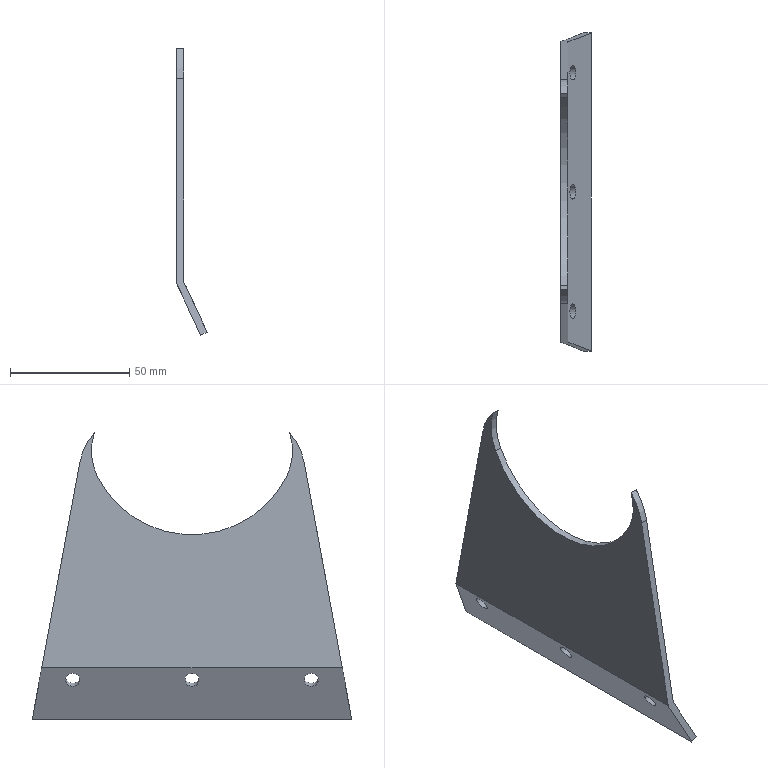Part | STEP file | 1-57.4 | 1 solid | 15 faces | box 12.749 x 134.024 x 120.156 mm | volume 31818 mm3 | cylinder 8 | plane 7 | commonest cylinder face diameters 6 x3 48 x2 51.19 x2 89 x1
STEP:
#1=CARTESIAN_POINT('',(0.,0.,0.));
#2=DIRECTION('',(0.,0.,1.));
#3=DIRECTION('',(1.,0.,0.));
#4=AXIS2_PLACEMENT_3D('',#1,#2,#3);
#5=CARTESIAN_POINT('',(0.,47.074,4.632));
#6=VERTEX_POINT('',#5);
#7=CARTESIAN_POINT('',(3.,47.074,4.632));
#8=VERTEX_POINT('',#7);
#9=CARTESIAN_POINT('',(0.,47.074,4.632));
#10=DIRECTION('',(1.,0.,0.));
#11=VECTOR('',#10,1.);
#12=LINE('',#9,#11);
#13=CARTESIAN_POINT('',(0.,57.043,-49.216));
#14=DIRECTION('',(0.,0.9833,0.182));
#15=DIRECTION('',(0.,-0.182,0.9833));
#16=AXIS2_PLACEMENT_3D('',#13,#14,#15);
#17=PLANE('',#16);
#18=CARTESIAN_POINT('',(54.763,0.));
#19=DIRECTION('',(0.,1.));
#20=VECTOR('',#19,1.);
#21=LINE('',#18,#20);
#22=(GEOMETRIC_REPRESENTATION_CONTEXT(2)PARAMETRIC_REPRESENTATION_CONTEXT()REPRESENTATION_CONTEXT('',''));
#23=DEFINITIONAL_REPRESENTATION('',(#21),#22);
#24=PCURVE('',#17,#23);
#25=CARTESIAN_POINT('',(-80.,21.907,-0.02707));
#26=DIRECTION('',(1.,0.,0.));
#27=DIRECTION('',(0.,0.9833,0.182));
#28=AXIS2_PLACEMENT_3D('',#25,#26,#27);
#29=CYLINDRICAL_SURFACE('',#28,25.595);
#30=CARTESIAN_POINT('',(0.,80.));
#31=DIRECTION('',(0.,1.));
#32=VECTOR('',#31,1.);
#33=LINE('',#30,#32);
#34=(GEOMETRIC_REPRESENTATION_CONTEXT(2)PARAMETRIC_REPRESENTATION_CONTEXT()REPRESENTATION_CONTEXT('',''));
#35=DEFINITIONAL_REPRESENTATION('',(#33),#34);
#36=PCURVE('',#29,#35);
#37=SURFACE_CURVE('',#12,(#24,#36),.PCURVE_S1.);
#38=EDGE_CURVE('',#6,#8,#37,.T.);
#39=ORIENTED_EDGE('',*,*,#38,.T.);
#40=CARTESIAN_POINT('',(3.,62.907,-80.889));
#41=VERTEX_POINT('',#40);
#42=CARTESIAN_POINT('',(3.,47.074,4.632));
#43=DIRECTION('',(0.,0.182,-0.9833));
#44=VECTOR('',#43,1.);
#45=LINE('',#42,#44);
#46=CARTESIAN_POINT('',(54.763,3.));
#47=DIRECTION('',(-1.,0.));
#48=VECTOR('',#47,1.);
#49=LINE('',#46,#48);
#50=(GEOMETRIC_REPRESENTATION_CONTEXT(2)PARAMETRIC_REPRESENTATION_CONTEXT()REPRESENTATION_CONTEXT('',''));
#51=DEFINITIONAL_REPRESENTATION('',(#49),#50);
#52=PCURVE('',#17,#51);
#53=CARTESIAN_POINT('',(3.,0.,-21.008));
#54=DIRECTION('',(-1.,0.,0.));
#55=DIRECTION('',(0.,0.,1.));
#56=AXIS2_PLACEMENT_3D('',#53,#54,#55);
#57=PLANE('',#56);
#58=CARTESIAN_POINT('',(25.64,47.074));
#59=DIRECTION('',(-0.9833,0.182));
#60=VECTOR('',#59,1.);
#61=LINE('',#58,#60);
#62=(GEOMETRIC_REPRESENTATION_CONTEXT(2)PARAMETRIC_REPRESENTATION_CONTEXT()REPRESENTATION_CONTEXT('',''));
#63=DEFINITIONAL_REPRESENTATION('',(#61),#62);
#64=PCURVE('',#57,#63);
#65=SURFACE_CURVE('',#45,(#52,#64),.PCURVE_S1.);
#66=EDGE_CURVE('',#8,#41,#65,.T.);
#67=ORIENTED_EDGE('',*,*,#66,.T.);
#68=CARTESIAN_POINT('',(12.749,66.777,-101.796));
#69=VERTEX_POINT('',#68);
#70=CARTESIAN_POINT('',(3.,62.907,-80.889));
#71=DIRECTION('',(0.4168,0.1655,-0.8938));
#72=VECTOR('',#71,1.);
#73=LINE('',#70,#72);
#74=CARTESIAN_POINT('',(-32.211,3.));
#75=DIRECTION('',(-0.909,0.4168));
#76=VECTOR('',#75,1.);
#77=LINE('',#74,#76);
#78=(GEOMETRIC_REPRESENTATION_CONTEXT(2)PARAMETRIC_REPRESENTATION_CONTEXT()REPRESENTATION_CONTEXT('',''));
#79=DEFINITIONAL_REPRESENTATION('',(#77),#78);
#80=PCURVE('',#17,#79);
#81=CARTESIAN_POINT('',(7.875,0.,-91.342));
#82=DIRECTION('',(-0.9063,0.,-0.4226));
#83=DIRECTION('',(-0.4226,0.,0.9063));
#84=AXIS2_PLACEMENT_3D('',#81,#82,#83);
#85=PLANE('',#84);
#86=CARTESIAN_POINT('',(11.534,62.907));
#87=DIRECTION('',(-0.9862,0.1655));
#88=VECTOR('',#87,1.);
#89=LINE('',#86,#88);
#90=(GEOMETRIC_REPRESENTATION_CONTEXT(2)PARAMETRIC_REPRESENTATION_CONTEXT()REPRESENTATION_CONTEXT('',''));
#91=DEFINITIONAL_REPRESENTATION('',(#89),#90);
#92=PCURVE('',#85,#91);
#93=SURFACE_CURVE('',#73,(#80,#92),.PCURVE_S1.);
#94=EDGE_CURVE('',#41,#69,#93,.T.);
#95=ORIENTED_EDGE('',*,*,#94,.T.);
#96=CARTESIAN_POINT('',(10.03,67.012,-103.064));
#97=VERTEX_POINT('',#96);
#98=CARTESIAN_POINT('',(12.749,66.777,-101.796));
#99=DIRECTION('',(-0.9035,0.078,-0.4213));
#100=VECTOR('',#99,1.);
#101=LINE('',#98,#100);
#102=CARTESIAN_POINT('',(-53.473,12.749));
#103=DIRECTION('',(-0.4285,-0.9035));
#104=VECTOR('',#103,1.);
#105=LINE('',#102,#104);
#106=(GEOMETRIC_REPRESENTATION_CONTEXT(2)PARAMETRIC_REPRESENTATION_CONTEXT()REPRESENTATION_CONTEXT('',''));
#107=DEFINITIONAL_REPRESENTATION('',(#105),#106);
#108=PCURVE('',#17,#107);
#109=CARTESIAN_POINT('',(11.39,0.,-102.43));
#110=DIRECTION('',(-0.4226,0.,0.9063));
#111=DIRECTION('',(0.9063,0.,0.4226));
#112=AXIS2_PLACEMENT_3D('',#109,#110,#111);
#113=PLANE('',#112);
#114=CARTESIAN_POINT('',(1.5,66.777));
#115=DIRECTION('',(-0.997,0.078));
#116=VECTOR('',#115,1.);
#117=LINE('',#114,#116);
#118=(GEOMETRIC_REPRESENTATION_CONTEXT(2)PARAMETRIC_REPRESENTATION_CONTEXT()REPRESENTATION_CONTEXT('',''));
#119=DEFINITIONAL_REPRESENTATION('',(#117),#118);
#120=PCURVE('',#113,#119);
#121=SURFACE_CURVE('',#101,(#108,#120),.PCURVE_S1.);
#122=EDGE_CURVE('',#69,#97,#121,.T.);
#123=ORIENTED_EDGE('',*,*,#122,.T.);
#124=CARTESIAN_POINT('',(0.,63.03,-81.554));
#125=VERTEX_POINT('',#124);
#126=CARTESIAN_POINT('',(10.03,67.012,-103.064));
#127=DIRECTION('',(-0.4168,-0.1655,0.8938));
#128=VECTOR('',#127,1.);
#129=LINE('',#126,#128);
#130=CARTESIAN_POINT('',(-54.763,10.03));
#131=DIRECTION('',(0.909,-0.4168));
#132=VECTOR('',#131,1.);
#133=LINE('',#130,#132);
#134=(GEOMETRIC_REPRESENTATION_CONTEXT(2)PARAMETRIC_REPRESENTATION_CONTEXT()REPRESENTATION_CONTEXT('',''));
#135=DEFINITIONAL_REPRESENTATION('',(#133),#134);
#136=PCURVE('',#17,#135);
#137=CARTESIAN_POINT('',(5.015,0.,-92.309));
#138=DIRECTION('',(0.9063,0.,0.4226));
#139=DIRECTION('',(0.4226,0.,-0.9063));
#140=AXIS2_PLACEMENT_3D('',#137,#138,#139);
#141=PLANE('',#140);
#142=CARTESIAN_POINT('',(11.867,67.012));
#143=DIRECTION('',(-0.9862,-0.1655));
#144=VECTOR('',#143,1.);
#145=LINE('',#142,#144);
#146=(GEOMETRIC_REPRESENTATION_CONTEXT(2)PARAMETRIC_REPRESENTATION_CONTEXT()REPRESENTATION_CONTEXT('',''));
#147=DEFINITIONAL_REPRESENTATION('',(#145),#146);
#148=PCURVE('',#141,#147);
#149=SURFACE_CURVE('',#129,(#136,#148),.PCURVE_S1.);
#150=EDGE_CURVE('',#97,#125,#149,.T.);
#151=ORIENTED_EDGE('',*,*,#150,.T.);
#152=CARTESIAN_POINT('',(0.,63.03,-81.554));
#153=DIRECTION('',(0.,-0.182,0.9833));
#154=VECTOR('',#153,1.);
#155=LINE('',#152,#154);
#156=CARTESIAN_POINT('',(-32.888,0.));
#157=DIRECTION('',(1.,0.));
#158=VECTOR('',#157,1.);
#159=LINE('',#156,#158);
#160=(GEOMETRIC_REPRESENTATION_CONTEXT(2)PARAMETRIC_REPRESENTATION_CONTEXT()REPRESENTATION_CONTEXT('',''));
#161=DEFINITIONAL_REPRESENTATION('',(#159),#160);
#162=PCURVE('',#17,#161);
#163=CARTESIAN_POINT('',(0.,0.,-21.341));
#164=DIRECTION('',(1.,0.,0.));
#165=DIRECTION('',(0.,0.,-1.));
#166=AXIS2_PLACEMENT_3D('',#163,#164,#165);
#167=PLANE('',#166);
#168=CARTESIAN_POINT('',(60.213,63.03));
#169=DIRECTION('',(-0.9833,-0.182));
#170=VECTOR('',#169,1.);
#171=LINE('',#168,#170);
#172=(GEOMETRIC_REPRESENTATION_CONTEXT(2)PARAMETRIC_REPRESENTATION_CONTEXT()REPRESENTATION_CONTEXT('',''));
#173=DEFINITIONAL_REPRESENTATION('',(#171),#172);
#174=PCURVE('',#167,#173);
#175=SURFACE_CURVE('',#155,(#162,#174),.PCURVE_S1.);
#176=EDGE_CURVE('',#125,#6,#175,.T.);
#177=ORIENTED_EDGE('',*,*,#176,.T.);
#178=EDGE_LOOP('',(#39,#67,#95,#123,#151,#177));
#179=FACE_BOUND('',#178,.T.);
#180=ADVANCED_FACE('',(#179),#17,.T.);
#181=CARTESIAN_POINT('',(0.,40.934,17.092));
#182=VERTEX_POINT('',#181);
#183=CARTESIAN_POINT('',(3.,40.934,17.092));
#184=VERTEX_POINT('',#183);
#185=CARTESIAN_POINT('',(0.,40.934,17.092));
#186=DIRECTION('',(1.,0.,0.));
#187=VECTOR('',#186,1.);
#188=LINE('',#185,#187);
#189=CARTESIAN_POINT('',(0.5496,80.));
#190=DIRECTION('',(0.,1.));
#191=VECTOR('',#190,1.);
#192=LINE('',#189,#191);
#193=(GEOMETRIC_REPRESENTATION_CONTEXT(2)PARAMETRIC_REPRESENTATION_CONTEXT()REPRESENTATION_CONTEXT('',''));
#194=DEFINITIONAL_REPRESENTATION('',(#192),#193);
#195=PCURVE('',#29,#194);
#196=CARTESIAN_POINT('',(167.5,18.2,9.4));
#197=DIRECTION('',(-1.,0.,0.));
#198=DIRECTION('',(0.,0.8878,-0.4602));
#199=AXIS2_PLACEMENT_3D('',#196,#197,#198);
#200=CYLINDRICAL_SURFACE('',#199,24.);
#201=CARTESIAN_POINT('',(5.479,167.5));
#202=DIRECTION('',(0.,-1.));
#203=VECTOR('',#202,1.);
#204=LINE('',#201,#203);
#205=(GEOMETRIC_REPRESENTATION_CONTEXT(2)PARAMETRIC_REPRESENTATION_CONTEXT()REPRESENTATION_CONTEXT('',''));
#206=DEFINITIONAL_REPRESENTATION('',(#204),#205);
#207=PCURVE('',#200,#206);
#208=SURFACE_CURVE('',#188,(#195,#207),.PCURVE_S1.);
#209=EDGE_CURVE('',#182,#184,#208,.T.);
#210=ORIENTED_EDGE('',*,*,#209,.T.);
#211=CARTESIAN_POINT('',(3.,21.907,-0.02707));
#212=DIRECTION('',(-1.,0.,0.));
#213=DIRECTION('',(0.,0.7434,0.6688));
#214=AXIS2_PLACEMENT_3D('',#211,#212,#213);
#215=CIRCLE('',#214,25.595);
#216=CARTESIAN_POINT('',(0.5496,83.));
#217=DIRECTION('',(-1.,0.));
#218=VECTOR('',#217,1.);
#219=LINE('',#216,#218);
#220=(GEOMETRIC_REPRESENTATION_CONTEXT(2)PARAMETRIC_REPRESENTATION_CONTEXT()REPRESENTATION_CONTEXT('',''));
#221=DEFINITIONAL_REPRESENTATION('',(#219),#220);
#222=PCURVE('',#29,#221);
#223=CARTESIAN_POINT('',(20.981,21.907));
#224=DIRECTION('',(0.6688,0.7434));
#225=AXIS2_PLACEMENT_2D('',#223,#224);
#226=CIRCLE('',#225,25.595);
#227=(GEOMETRIC_REPRESENTATION_CONTEXT(2)PARAMETRIC_REPRESENTATION_CONTEXT()REPRESENTATION_CONTEXT('',''));
#228=DEFINITIONAL_REPRESENTATION('',(#226),#227);
#229=PCURVE('',#57,#228);
#230=SURFACE_CURVE('',#215,(#222,#229),.PCURVE_S1.);
#231=EDGE_CURVE('',#184,#8,#230,.T.);
#232=ORIENTED_EDGE('',*,*,#231,.T.);
#233=ORIENTED_EDGE('',*,*,#38,.F.);
#234=CARTESIAN_POINT('',(0.,21.907,-0.02707));
#235=DIRECTION('',(1.,0.,0.));
#236=DIRECTION('',(0.,0.9833,0.182));
#237=AXIS2_PLACEMENT_3D('',#234,#235,#236);
#238=CIRCLE('',#237,25.595);
#239=CARTESIAN_POINT('',(0.,80.));
#240=DIRECTION('',(1.,0.));
#241=VECTOR('',#240,1.);
#242=LINE('',#239,#241);
#243=(GEOMETRIC_REPRESENTATION_CONTEXT(2)PARAMETRIC_REPRESENTATION_CONTEXT()REPRESENTATION_CONTEXT('',''));
#244=DEFINITIONAL_REPRESENTATION('',(#242),#243);
#245=PCURVE('',#29,#244);
#246=CARTESIAN_POINT('',(-21.314,21.907));
#247=DIRECTION('',(-0.182,0.9833));
#248=AXIS2_PLACEMENT_2D('',#246,#247);
#249=CIRCLE('',#248,25.595);
#250=(GEOMETRIC_REPRESENTATION_CONTEXT(2)PARAMETRIC_REPRESENTATION_CONTEXT()REPRESENTATION_CONTEXT('',''));
#251=DEFINITIONAL_REPRESENTATION('',(#249),#250);
#252=PCURVE('',#167,#251);
#253=SURFACE_CURVE('',#238,(#245,#252),.PCURVE_S1.);
#254=EDGE_CURVE('',#6,#182,#253,.T.);
#255=ORIENTED_EDGE('',*,*,#254,.T.);
#256=EDGE_LOOP('',(#210,#232,#233,#255));
#257=FACE_BOUND('',#256,.T.);
#258=ADVANCED_FACE('',(#257),#29,.T.);
#259=CARTESIAN_POINT('',(0.,-40.934,17.092));
#260=VERTEX_POINT('',#259);
#261=CARTESIAN_POINT('',(3.,-40.934,17.092));
#262=VERTEX_POINT('',#261);
#263=CARTESIAN_POINT('',(0.,-40.934,17.092));
#264=DIRECTION('',(1.,0.,0.));
#265=VECTOR('',#264,1.);
#266=LINE('',#263,#265);
#267=CARTESIAN_POINT('',(-80.,-21.907,-0.02707));
#268=DIRECTION('',(1.,0.,0.));
#269=DIRECTION('',(0.,-0.7434,0.6688));
#270=AXIS2_PLACEMENT_3D('',#267,#268,#269);
#271=CYLINDRICAL_SURFACE('',#270,25.595);
#272=CARTESIAN_POINT('',(0.,80.));
#273=DIRECTION('',(0.,1.));
#274=VECTOR('',#273,1.);
#275=LINE('',#272,#274);
#276=(GEOMETRIC_REPRESENTATION_CONTEXT(2)PARAMETRIC_REPRESENTATION_CONTEXT()REPRESENTATION_CONTEXT('',''));
#277=DEFINITIONAL_REPRESENTATION('',(#275),#276);
#278=PCURVE('',#271,#277);
#279=CARTESIAN_POINT('',(167.5,-18.2,9.4));
#280=DIRECTION('',(-1.,0.,0.));
#281=DIRECTION('',(0.,-0.5515,0.8342));
#282=AXIS2_PLACEMENT_3D('',#279,#280,#281);
#283=CYLINDRICAL_SURFACE('',#282,24.);
#284=CARTESIAN_POINT('',(5.623,167.5));
#285=DIRECTION('',(0.,-1.));
#286=VECTOR('',#285,1.);
#287=LINE('',#284,#286);
#288=(GEOMETRIC_REPRESENTATION_CONTEXT(2)PARAMETRIC_REPRESENTATION_CONTEXT()REPRESENTATION_CONTEXT('',''));
#289=DEFINITIONAL_REPRESENTATION('',(#287),#288);
#290=PCURVE('',#283,#289);
#291=SURFACE_CURVE('',#266,(#278,#290),.PCURVE_S1.);
#292=EDGE_CURVE('',#260,#262,#291,.T.);
#293=ORIENTED_EDGE('',*,*,#292,.F.);
#294=CARTESIAN_POINT('',(0.,-47.074,4.632));
#295=VERTEX_POINT('',#294);
#296=CARTESIAN_POINT('',(0.,-21.907,-0.02707));
#297=DIRECTION('',(1.,0.,0.));
#298=DIRECTION('',(0.,-0.7434,0.6688));
#299=AXIS2_PLACEMENT_3D('',#296,#297,#298);
#300=CIRCLE('',#299,25.595);
#301=CARTESIAN_POINT('',(0.,80.));
#302=DIRECTION('',(1.,0.));
#303=VECTOR('',#302,1.);
#304=LINE('',#301,#303);
#305=(GEOMETRIC_REPRESENTATION_CONTEXT(2)PARAMETRIC_REPRESENTATION_CONTEXT()REPRESENTATION_CONTEXT('',''));
#306=DEFINITIONAL_REPRESENTATION('',(#304),#305);
#307=PCURVE('',#271,#306);
#308=CARTESIAN_POINT('',(-21.314,-21.907));
#309=DIRECTION('',(-0.6688,-0.7434));
#310=AXIS2_PLACEMENT_2D('',#308,#309);
#311=CIRCLE('',#310,25.595);
#312=(GEOMETRIC_REPRESENTATION_CONTEXT(2)PARAMETRIC_REPRESENTATION_CONTEXT()REPRESENTATION_CONTEXT('',''));
#313=DEFINITIONAL_REPRESENTATION('',(#311),#312);
#314=PCURVE('',#167,#313);
#315=SURFACE_CURVE('',#300,(#307,#314),.PCURVE_S1.);
#316=EDGE_CURVE('',#260,#295,#315,.T.);
#317=ORIENTED_EDGE('',*,*,#316,.T.);
#318=CARTESIAN_POINT('',(3.,-47.074,4.632));
#319=VERTEX_POINT('',#318);
#320=CARTESIAN_POINT('',(0.,-47.074,4.632));
#321=DIRECTION('',(1.,0.,0.));
#322=VECTOR('',#321,1.);
#323=LINE('',#320,#322);
#324=CARTESIAN_POINT('',(0.5496,80.));
#325=DIRECTION('',(0.,1.));
#326=VECTOR('',#325,1.);
#327=LINE('',#324,#326);
#328=(GEOMETRIC_REPRESENTATION_CONTEXT(2)PARAMETRIC_REPRESENTATION_CONTEXT()REPRESENTATION_CONTEXT('',''));
#329=DEFINITIONAL_REPRESENTATION('',(#327),#328);
#330=PCURVE('',#271,#329);
#331=CARTESIAN_POINT('',(0.,-57.043,-49.216));
#332=DIRECTION('',(0.,-0.9833,0.182));
#333=DIRECTION('',(0.,-0.182,-0.9833));
#334=AXIS2_PLACEMENT_3D('',#331,#332,#333);
#335=PLANE('',#334);
#336=CARTESIAN_POINT('',(-54.763,0.));
#337=DIRECTION('',(0.,1.));
#338=VECTOR('',#337,1.);
#339=LINE('',#336,#338);
#340=(GEOMETRIC_REPRESENTATION_CONTEXT(2)PARAMETRIC_REPRESENTATION_CONTEXT()REPRESENTATION_CONTEXT('',''));
#341=DEFINITIONAL_REPRESENTATION('',(#339),#340);
#342=PCURVE('',#335,#341);
#343=SURFACE_CURVE('',#323,(#330,#342),.PCURVE_S1.);
#344=EDGE_CURVE('',#295,#319,#343,.T.);
#345=ORIENTED_EDGE('',*,*,#344,.T.);
#346=CARTESIAN_POINT('',(3.,-21.907,-0.02707));
#347=DIRECTION('',(-1.,0.,0.));
#348=DIRECTION('',(0.,-0.9833,0.182));
#349=AXIS2_PLACEMENT_3D('',#346,#347,#348);
#350=CIRCLE('',#349,25.595);
#351=CARTESIAN_POINT('',(0.5496,83.));
#352=DIRECTION('',(-1.,0.));
#353=VECTOR('',#352,1.);
#354=LINE('',#351,#353);
#355=(GEOMETRIC_REPRESENTATION_CONTEXT(2)PARAMETRIC_REPRESENTATION_CONTEXT()REPRESENTATION_CONTEXT('',''));
#356=DEFINITIONAL_REPRESENTATION('',(#354),#355);
#357=PCURVE('',#271,#356);
#358=CARTESIAN_POINT('',(20.981,-21.907));
#359=DIRECTION('',(0.182,-0.9833));
#360=AXIS2_PLACEMENT_2D('',#358,#359);
#361=CIRCLE('',#360,25.595);
#362=(GEOMETRIC_REPRESENTATION_CONTEXT(2)PARAMETRIC_REPRESENTATION_CONTEXT()REPRESENTATION_CONTEXT('',''));
#363=DEFINITIONAL_REPRESENTATION('',(#361),#362);
#364=PCURVE('',#57,#363);
#365=SURFACE_CURVE('',#350,(#357,#364),.PCURVE_S1.);
#366=EDGE_CURVE('',#319,#262,#365,.T.);
#367=ORIENTED_EDGE('',*,*,#366,.T.);
#368=EDGE_LOOP('',(#293,#317,#345,#367));
#369=FACE_BOUND('',#368,.T.);
#370=ADVANCED_FACE('',(#369),#271,.T.);
#371=ORIENTED_EDGE('',*,*,#344,.F.);
#372=CARTESIAN_POINT('',(0.,-63.03,-81.554));
#373=VERTEX_POINT('',#372);
#374=CARTESIAN_POINT('',(0.,-47.074,4.632));
#375=DIRECTION('',(0.,-0.182,-0.9833));
#376=VECTOR('',#375,1.);
#377=LINE('',#374,#376);
#378=CARTESIAN_POINT('',(-54.763,0.));
#379=DIRECTION('',(1.,0.));
#380=VECTOR('',#379,1.);
#381=LINE('',#378,#380);
#382=(GEOMETRIC_REPRESENTATION_CONTEXT(2)PARAMETRIC_REPRESENTATION_CONTEXT()REPRESENTATION_CONTEXT('',''));
#383=DEFINITIONAL_REPRESENTATION('',(#381),#382);
#384=PCURVE('',#335,#383);
#385=CARTESIAN_POINT('',(-25.973,-47.074));
#386=DIRECTION('',(0.9833,-0.182));
#387=VECTOR('',#386,1.);
#388=LINE('',#385,#387);
#389=(GEOMETRIC_REPRESENTATION_CONTEXT(2)PARAMETRIC_REPRESENTATION_CONTEXT()REPRESENTATION_CONTEXT('',''));
#390=DEFINITIONAL_REPRESENTATION('',(#388),#389);
#391=PCURVE('',#167,#390);
#392=SURFACE_CURVE('',#377,(#384,#391),.PCURVE_S1.);
#393=EDGE_CURVE('',#295,#373,#392,.T.);
#394=ORIENTED_EDGE('',*,*,#393,.T.);
#395=CARTESIAN_POINT('',(10.03,-67.012,-103.064));
#396=VERTEX_POINT('',#395);
#397=CARTESIAN_POINT('',(0.,-63.03,-81.554));
#398=DIRECTION('',(0.4168,-0.1655,-0.8938));
#399=VECTOR('',#398,1.);
#400=LINE('',#397,#399);
#401=CARTESIAN_POINT('',(32.888,0.));
#402=DIRECTION('',(0.909,0.4168));
#403=VECTOR('',#402,1.);
#404=LINE('',#401,#403);
#405=(GEOMETRIC_REPRESENTATION_CONTEXT(2)PARAMETRIC_REPRESENTATION_CONTEXT()REPRESENTATION_CONTEXT('',''));
#406=DEFINITIONAL_REPRESENTATION('',(#404),#405);
#407=PCURVE('',#335,#406);
#408=CARTESIAN_POINT('',(-11.867,-63.03));
#409=DIRECTION('',(0.9862,-0.1655));
#410=VECTOR('',#409,1.);
#411=LINE('',#408,#410);
#412=(GEOMETRIC_REPRESENTATION_CONTEXT(2)PARAMETRIC_REPRESENTATION_CONTEXT()REPRESENTATION_CONTEXT('',''));
#413=DEFINITIONAL_REPRESENTATION('',(#411),#412);
#414=PCURVE('',#141,#413);
#415=SURFACE_CURVE('',#400,(#407,#414),.PCURVE_S1.);
#416=EDGE_CURVE('',#373,#396,#415,.T.);
#417=ORIENTED_EDGE('',*,*,#416,.T.);
#418=CARTESIAN_POINT('',(12.749,-66.777,-101.796));
#419=VERTEX_POINT('',#418);
#420=CARTESIAN_POINT('',(10.03,-67.012,-103.064));
#421=DIRECTION('',(0.9035,0.078,0.4213));
#422=VECTOR('',#421,1.);
#423=LINE('',#420,#422);
#424=CARTESIAN_POINT('',(54.763,10.03));
#425=DIRECTION('',(-0.4285,0.9035));
#426=VECTOR('',#425,1.);
#427=LINE('',#424,#426);
#428=(GEOMETRIC_REPRESENTATION_CONTEXT(2)PARAMETRIC_REPRESENTATION_CONTEXT()REPRESENTATION_CONTEXT('',''));
#429=DEFINITIONAL_REPRESENTATION('',(#427),#428);
#430=PCURVE('',#335,#429);
#431=CARTESIAN_POINT('',(-1.5,-67.012));
#432=DIRECTION('',(0.997,0.078));
#433=VECTOR('',#432,1.);
#434=LINE('',#431,#433);
#435=(GEOMETRIC_REPRESENTATION_CONTEXT(2)PARAMETRIC_REPRESENTATION_CONTEXT()REPRESENTATION_CONTEXT('',''));
#436=DEFINITIONAL_REPRESENTATION('',(#434),#435);
#437=PCURVE('',#113,#436);
#438=SURFACE_CURVE('',#423,(#430,#437),.PCURVE_S1.);
#439=EDGE_CURVE('',#396,#419,#438,.T.);
#440=ORIENTED_EDGE('',*,*,#439,.T.);
#441=CARTESIAN_POINT('',(3.,-62.907,-80.889));
#442=VERTEX_POINT('',#441);
#443=CARTESIAN_POINT('',(12.749,-66.777,-101.796));
#444=DIRECTION('',(-0.4168,0.1655,0.8938));
#445=VECTOR('',#444,1.);
#446=LINE('',#443,#445);
#447=CARTESIAN_POINT('',(53.473,12.749));
#448=DIRECTION('',(-0.909,-0.4168));
#449=VECTOR('',#448,1.);
#450=LINE('',#447,#449);
#451=(GEOMETRIC_REPRESENTATION_CONTEXT(2)PARAMETRIC_REPRESENTATION_CONTEXT()REPRESENTATION_CONTEXT('',''));
#452=DEFINITIONAL_REPRESENTATION('',(#450),#451);
#453=PCURVE('',#335,#452);
#454=CARTESIAN_POINT('',(-11.534,-66.777));
#455=DIRECTION('',(0.9862,0.1655));
#456=VECTOR('',#455,1.);
#457=LINE('',#454,#456);
#458=(GEOMETRIC_REPRESENTATION_CONTEXT(2)PARAMETRIC_REPRESENTATION_CONTEXT()REPRESENTATION_CONTEXT('',''));
#459=DEFINITIONAL_REPRESENTATION('',(#457),#458);
#460=PCURVE('',#85,#459);
#461=SURFACE_CURVE('',#446,(#453,#460),.PCURVE_S1.);
#462=EDGE_CURVE('',#419,#442,#461,.T.);
#463=ORIENTED_EDGE('',*,*,#462,.T.);
#464=CARTESIAN_POINT('',(3.,-62.907,-80.889));
#465=DIRECTION('',(0.,0.182,0.9833));
#466=VECTOR('',#465,1.);
#467=LINE('',#464,#466);
#468=CARTESIAN_POINT('',(32.211,3.));
#469=DIRECTION('',(-1.,0.));
#470=VECTOR('',#469,1.);
#471=LINE('',#468,#470);
#472=(GEOMETRIC_REPRESENTATION_CONTEXT(2)PARAMETRIC_REPRESENTATION_CONTEXT()REPRESENTATION_CONTEXT('',''));
#473=DEFINITIONAL_REPRESENTATION('',(#471),#472);
#474=PCURVE('',#335,#473);
#475=CARTESIAN_POINT('',(-59.881,-62.907));
#476=DIRECTION('',(0.9833,0.182));
#477=VECTOR('',#476,1.);
#478=LINE('',#475,#477);
#479=(GEOMETRIC_REPRESENTATION_CONTEXT(2)PARAMETRIC_REPRESENTATION_CONTEXT()REPRESENTATION_CONTEXT('',''));
#480=DEFINITIONAL_REPRESENTATION('',(#478),#479);
#481=PCURVE('',#57,#480);
#482=SURFACE_CURVE('',#467,(#474,#481),.PCURVE_S1.);
#483=EDGE_CURVE('',#442,#319,#482,.T.);
#484=ORIENTED_EDGE('',*,*,#483,.T.);
#485=EDGE_LOOP('',(#371,#394,#417,#440,#463,#484));
#486=FACE_BOUND('',#485,.T.);
#487=ADVANCED_FACE('',(#486),#335,.T.);
#488=CARTESIAN_POINT('',(12.749,-66.777,-101.796));
#489=DIRECTION('',(0.,1.,0.));
#490=VECTOR('',#489,1.);
#491=LINE('',#488,#490);
#492=CARTESIAN_POINT('',(1.5,-66.777));
#493=DIRECTION('',(0.,1.));
#494=VECTOR('',#493,1.);
#495=LINE('',#492,#494);
#496=(GEOMETRIC_REPRESENTATION_CONTEXT(2)PARAMETRIC_REPRESENTATION_CONTEXT()REPRESENTATION_CONTEXT('',''));
#497=DEFINITIONAL_REPRESENTATION('',(#495),#496);
#498=PCURVE('',#113,#497);
#499=CARTESIAN_POINT('',(-11.534,-66.777));
#500=DIRECTION('',(0.,1.));
#501=VECTOR('',#500,1.);
#502=LINE('',#499,#501);
#503=(GEOMETRIC_REPRESENTATION_CONTEXT(2)PARAMETRIC_REPRESENTATION_CONTEXT()REPRESENTATION_CONTEXT('',''));
#504=DEFINITIONAL_REPRESENTATION('',(#502),#503);
#505=PCURVE('',#85,#504);
#506=SURFACE_CURVE('',#491,(#498,#505),.PCURVE_S1.);
#507=EDGE_CURVE('',#419,#69,#506,.T.);
#508=ORIENTED_EDGE('',*,*,#507,.T.);
#509=ORIENTED_EDGE('',*,*,#122,.T.);
#510=CARTESIAN_POINT('',(10.03,-67.012,-103.064));
#511=DIRECTION('',(0.,1.,0.));
#512=VECTOR('',#511,1.);
#513=LINE('',#510,#512);
#514=CARTESIAN_POINT('',(-1.5,-67.012));
#515=DIRECTION('',(0.,1.));
#516=VECTOR('',#515,1.);
#517=LINE('',#514,#516);
#518=(GEOMETRIC_REPRESENTATION_CONTEXT(2)PARAMETRIC_REPRESENTATION_CONTEXT()REPRESENTATION_CONTEXT('',''));
#519=DEFINITIONAL_REPRESENTATION('',(#517),#518);
#520=PCURVE('',#113,#519);
#521=CARTESIAN_POINT('',(11.867,-67.012));
#522=DIRECTION('',(0.,1.));
#523=VECTOR('',#522,1.);
#524=LINE('',#521,#523);
#525=(GEOMETRIC_REPRESENTATION_CONTEXT(2)PARAMETRIC_REPRESENTATION_CONTEXT()REPRESENTATION_CONTEXT('',''));
#526=DEFINITIONAL_REPRESENTATION('',(#524),#525);
#527=PCURVE('',#141,#526);
#528=SURFACE_CURVE('',#513,(#520,#527),.PCURVE_S1.);
#529=EDGE_CURVE('',#396,#97,#528,.T.);
#530=ORIENTED_EDGE('',*,*,#529,.F.);
#531=ORIENTED_EDGE('',*,*,#439,.T.);
#532=EDGE_LOOP('',(#508,#509,#530,#531));
#533=FACE_BOUND('',#532,.F.);
#534=ADVANCED_FACE('',(#533),#113,.F.);
#535=CARTESIAN_POINT('',(3.,-62.907,-80.889));
#536=DIRECTION('',(0.,1.,0.));
#537=VECTOR('',#536,1.);
#538=LINE('',#535,#537);
#539=CARTESIAN_POINT('',(-59.881,-62.907));
#540=DIRECTION('',(0.,1.));
#541=VECTOR('',#540,1.);
#542=LINE('',#539,#541);
#543=(GEOMETRIC_REPRESENTATION_CONTEXT(2)PARAMETRIC_REPRESENTATION_CONTEXT()REPRESENTATION_CONTEXT('',''));
#544=DEFINITIONAL_REPRESENTATION('',(#542),#543);
#545=PCURVE('',#57,#544);
#546=CARTESIAN_POINT('',(11.534,-62.907));
#547=DIRECTION('',(0.,1.));
#548=VECTOR('',#547,1.);
#549=LINE('',#546,#548);
#550=(GEOMETRIC_REPRESENTATION_CONTEXT(2)PARAMETRIC_REPRESENTATION_CONTEXT()REPRESENTATION_CONTEXT('',''));
#551=DEFINITIONAL_REPRESENTATION('',(#549),#550);
#552=PCURVE('',#85,#551);
#553=SURFACE_CURVE('',#538,(#545,#552),.PCURVE_S1.);
#554=EDGE_CURVE('',#442,#41,#553,.T.);
#555=ORIENTED_EDGE('',*,*,#554,.F.);
#556=ORIENTED_EDGE('',*,*,#483,.T.);
#557=ORIENTED_EDGE('',*,*,#366,.T.);
#558=CARTESIAN_POINT('',(3.,-39.507,-1.645));
#559=VERTEX_POINT('',#558);
#560=CARTESIAN_POINT('',(3.,-18.2,9.4));
#561=DIRECTION('',(1.,0.,0.));
#562=DIRECTION('',(0.,-0.9472,0.3205));
#563=AXIS2_PLACEMENT_3D('',#560,#561,#562);
#564=CIRCLE('',#563,24.);
#565=CARTESIAN_POINT('',(38.1,-40.934));
#566=CARTESIAN_POINT('',(-1.276,-54.257));
#567=CARTESIAN_POINT('',(6.874,-13.495));
#568=CARTESIAN_POINT('',(15.024,27.268));
#569=CARTESIAN_POINT('',(46.25,-0.1715));
#570=CARTESIAN_POINT('',(77.477,-27.611));
#571=CARTESIAN_POINT('',(38.1,-40.934));
#572=(BOUNDED_CURVE()B_SPLINE_CURVE(2,(#565,#566,#567,#568,#569,#570,#571),.UNSPECIFIED.,.T.,.F.)B_SPLINE_CURVE_WITH_KNOTS((1,2,2,2,2,1),(-2.094,0.,2.094,4.189,6.283,8.378),.UNSPECIFIED.)CURVE()GEOMETRIC_REPRESENTATION_ITEM()RATIONAL_B_SPLINE_CURVE((1.,0.5,1.,0.5,1.,0.5,1.))REPRESENTATION_ITEM(''));
#573=(GEOMETRIC_REPRESENTATION_CONTEXT(2)PARAMETRIC_REPRESENTATION_CONTEXT()REPRESENTATION_CONTEXT('',''));
#574=DEFINITIONAL_REPRESENTATION('',(#572),#573);
#575=PCURVE('',#57,#574);
#576=CARTESIAN_POINT('',(5.623,164.5));
#577=DIRECTION('',(-1.,0.));
#578=VECTOR('',#577,1.);
#579=LINE('',#576,#578);
#580=(GEOMETRIC_REPRESENTATION_CONTEXT(2)PARAMETRIC_REPRESENTATION_CONTEXT()REPRESENTATION_CONTEXT('',''));
#581=DEFINITIONAL_REPRESENTATION('',(#579),#580);
#582=PCURVE('',#283,#581);
#583=SURFACE_CURVE('',#564,(#575,#582),.PCURVE_S1.);
#584=EDGE_CURVE('',#262,#559,#583,.T.);
#585=ORIENTED_EDGE('',*,*,#584,.T.);
#586=CARTESIAN_POINT('',(3.,39.507,-1.645));
#587=VERTEX_POINT('',#586);
#588=CARTESIAN_POINT('',(3.,0.,18.835));
#589=DIRECTION('',(1.,0.,0.));
#590=DIRECTION('',(0.,-0.8878,-0.4602));
#591=AXIS2_PLACEMENT_3D('',#588,#589,#590);
#592=CIRCLE('',#591,44.5);
#593=CARTESIAN_POINT('',(19.363,-39.507));
#594=CARTESIAN_POINT('',(-49.066,-4.035));
#595=CARTESIAN_POINT('',(15.868,37.49));
#596=CARTESIAN_POINT('',(80.802,79.015));
#597=CARTESIAN_POINT('',(84.297,2.018));
#598=CARTESIAN_POINT('',(87.792,-74.979));
#599=CARTESIAN_POINT('',(19.363,-39.507));
#600=(BOUNDED_CURVE()B_SPLINE_CURVE(2,(#593,#594,#595,#596,#597,#598,#599),.UNSPECIFIED.,.T.,.F.)B_SPLINE_CURVE_WITH_KNOTS((1,2,2,2,2,1),(-2.094,0.,2.094,4.189,6.283,8.378),.UNSPECIFIED.)CURVE()GEOMETRIC_REPRESENTATION_ITEM()RATIONAL_B_SPLINE_CURVE((1.,0.5,1.,0.5,1.,0.5,1.))REPRESENTATION_ITEM(''));
#601=(GEOMETRIC_REPRESENTATION_CONTEXT(2)PARAMETRIC_REPRESENTATION_CONTEXT()REPRESENTATION_CONTEXT('',''));
#602=DEFINITIONAL_REPRESENTATION('',(#600),#601);
#603=PCURVE('',#57,#602);
#604=CARTESIAN_POINT('',(167.5,0.,18.835));
#605=DIRECTION('',(-1.,0.,0.));
#606=DIRECTION('',(0.,-0.8878,-0.4602));
#607=AXIS2_PLACEMENT_3D('',#604,#605,#606);
#608=CYLINDRICAL_SURFACE('',#607,44.5);
#609=CARTESIAN_POINT('',(6.283,164.5));
#610=DIRECTION('',(-1.,0.));
#611=VECTOR('',#610,1.);
#612=LINE('',#609,#611);
#613=(GEOMETRIC_REPRESENTATION_CONTEXT(2)PARAMETRIC_REPRESENTATION_CONTEXT()REPRESENTATION_CONTEXT('',''));
#614=DEFINITIONAL_REPRESENTATION('',(#612),#613);
#615=PCURVE('',#608,#614);
#616=SURFACE_CURVE('',#592,(#603,#615),.PCURVE_S1.);
#617=EDGE_CURVE('',#559,#587,#616,.T.);
#618=ORIENTED_EDGE('',*,*,#617,.T.);
#619=CARTESIAN_POINT('',(3.,18.2,9.4));
#620=DIRECTION('',(1.,0.,0.));
#621=DIRECTION('',(0.,0.8878,-0.4602));
#622=AXIS2_PLACEMENT_3D('',#619,#620,#621);
#623=CIRCLE('',#622,24.);
#624=CARTESIAN_POINT('',(19.363,39.507));
#625=CARTESIAN_POINT('',(56.268,58.638));
#626=CARTESIAN_POINT('',(54.383,17.112));
#627=CARTESIAN_POINT('',(52.499,-24.415));
#628=CARTESIAN_POINT('',(17.478,-2.019));
#629=CARTESIAN_POINT('',(-17.542,20.376));
#630=CARTESIAN_POINT('',(19.363,39.507));
#631=(BOUNDED_CURVE()B_SPLINE_CURVE(2,(#624,#625,#626,#627,#628,#629,#630),.UNSPECIFIED.,.T.,.F.)B_SPLINE_CURVE_WITH_KNOTS((1,2,2,2,2,1),(-2.094,0.,2.094,4.189,6.283,8.378),.UNSPECIFIED.)CURVE()GEOMETRIC_REPRESENTATION_ITEM()RATIONAL_B_SPLINE_CURVE((1.,0.5,1.,0.5,1.,0.5,1.))REPRESENTATION_ITEM(''));
#632=(GEOMETRIC_REPRESENTATION_CONTEXT(2)PARAMETRIC_REPRESENTATION_CONTEXT()REPRESENTATION_CONTEXT('',''));
#633=DEFINITIONAL_REPRESENTATION('',(#631),#632);
#634=PCURVE('',#57,#633);
#635=CARTESIAN_POINT('',(6.283,164.5));
#636=DIRECTION('',(-1.,0.));
#637=VECTOR('',#636,1.);
#638=LINE('',#635,#637);
#639=(GEOMETRIC_REPRESENTATION_CONTEXT(2)PARAMETRIC_REPRESENTATION_CONTEXT()REPRESENTATION_CONTEXT('',''));
#640=DEFINITIONAL_REPRESENTATION('',(#638),#639);
#641=PCURVE('',#200,#640);
#642=SURFACE_CURVE('',#623,(#634,#641),.PCURVE_S1.);
#643=EDGE_CURVE('',#587,#184,#642,.T.);
#644=ORIENTED_EDGE('',*,*,#643,.T.);
#645=ORIENTED_EDGE('',*,*,#231,.T.);
#646=ORIENTED_EDGE('',*,*,#66,.T.);
#647=EDGE_LOOP('',(#555,#556,#557,#585,#618,#644,#645,#646));
#648=FACE_BOUND('',#647,.F.);
#649=ADVANCED_FACE('',(#648),#57,.F.);
#650=CARTESIAN_POINT('',(0.,-63.03,-81.554));
#651=DIRECTION('',(0.,1.,0.));
#652=VECTOR('',#651,1.);
#653=LINE('',#650,#652);
#654=CARTESIAN_POINT('',(60.213,-63.03));
#655=DIRECTION('',(0.,1.));
#656=VECTOR('',#655,1.);
#657=LINE('',#654,#656);
#658=(GEOMETRIC_REPRESENTATION_CONTEXT(2)PARAMETRIC_REPRESENTATION_CONTEXT()REPRESENTATION_CONTEXT('',''));
#659=DEFINITIONAL_REPRESENTATION('',(#657),#658);
#660=PCURVE('',#167,#659);
#661=CARTESIAN_POINT('',(-11.867,-63.03));
#662=DIRECTION('',(0.,1.));
#663=VECTOR('',#662,1.);
#664=LINE('',#661,#663);
#665=(GEOMETRIC_REPRESENTATION_CONTEXT(2)PARAMETRIC_REPRESENTATION_CONTEXT()REPRESENTATION_CONTEXT('',''));
#666=DEFINITIONAL_REPRESENTATION('',(#664),#665);
#667=PCURVE('',#141,#666);
#668=SURFACE_CURVE('',#653,(#660,#667),.PCURVE_S1.);
#669=EDGE_CURVE('',#373,#125,#668,.T.);
#670=ORIENTED_EDGE('',*,*,#669,.T.);
#671=ORIENTED_EDGE('',*,*,#176,.T.);
#672=ORIENTED_EDGE('',*,*,#254,.T.);
#673=CARTESIAN_POINT('',(0.,39.507,-1.645));
#674=VERTEX_POINT('',#673);
#675=CARTESIAN_POINT('',(0.,18.2,9.4));
#676=DIRECTION('',(-1.,0.,0.));
#677=DIRECTION('',(0.,0.9472,0.3205));
#678=AXIS2_PLACEMENT_3D('',#675,#676,#677);
#679=CIRCLE('',#678,24.);
#680=CARTESIAN_POINT('',(-38.433,40.934));
#681=CARTESIAN_POINT('',(0.9436,54.257));
#682=CARTESIAN_POINT('',(-7.206,13.495));
#683=CARTESIAN_POINT('',(-15.357,-27.268));
#684=CARTESIAN_POINT('',(-46.583,0.1715));
#685=CARTESIAN_POINT('',(-77.809,27.611));
#686=CARTESIAN_POINT('',(-38.433,40.934));
#687=(BOUNDED_CURVE()B_SPLINE_CURVE(2,(#680,#681,#682,#683,#684,#685,#686),.UNSPECIFIED.,.T.,.F.)B_SPLINE_CURVE_WITH_KNOTS((1,2,2,2,2,1),(-2.094,0.,2.094,4.189,6.283,8.378),.UNSPECIFIED.)CURVE()GEOMETRIC_REPRESENTATION_ITEM()RATIONAL_B_SPLINE_CURVE((1.,0.5,1.,0.5,1.,0.5,1.))REPRESENTATION_ITEM(''));
#688=(GEOMETRIC_REPRESENTATION_CONTEXT(2)PARAMETRIC_REPRESENTATION_CONTEXT()REPRESENTATION_CONTEXT('',''));
#689=DEFINITIONAL_REPRESENTATION('',(#687),#688);
#690=PCURVE('',#167,#689);
#691=CARTESIAN_POINT('',(5.479,167.5));
#692=DIRECTION('',(1.,0.));
#693=VECTOR('',#692,1.);
#694=LINE('',#691,#693);
#695=(GEOMETRIC_REPRESENTATION_CONTEXT(2)PARAMETRIC_REPRESENTATION_CONTEXT()REPRESENTATION_CONTEXT('',''));
#696=DEFINITIONAL_REPRESENTATION('',(#694),#695);
#697=PCURVE('',#200,#696);
#698=SURFACE_CURVE('',#679,(#690,#697),.PCURVE_S1.);
#699=EDGE_CURVE('',#182,#674,#698,.T.);
#700=ORIENTED_EDGE('',*,*,#699,.T.);
#701=CARTESIAN_POINT('',(0.,-39.507,-1.645));
#702=VERTEX_POINT('',#701);
#703=CARTESIAN_POINT('',(0.,0.,18.835));
#704=DIRECTION('',(-1.,0.,0.));
#705=DIRECTION('',(0.,0.8878,-0.4602));
#706=AXIS2_PLACEMENT_3D('',#703,#704,#705);
#707=CIRCLE('',#706,44.5);
#708=CARTESIAN_POINT('',(-19.695,39.507));
#709=CARTESIAN_POINT('',(48.733,4.035));
#710=CARTESIAN_POINT('',(-16.201,-37.49));
#711=CARTESIAN_POINT('',(-81.135,-79.015));
#712=CARTESIAN_POINT('',(-84.629,-2.018));
#713=CARTESIAN_POINT('',(-88.124,74.979));
#714=CARTESIAN_POINT('',(-19.695,39.507));
#715=(BOUNDED_CURVE()B_SPLINE_CURVE(2,(#708,#709,#710,#711,#712,#713,#714),.UNSPECIFIED.,.T.,.F.)B_SPLINE_CURVE_WITH_KNOTS((1,2,2,2,2,1),(-2.094,0.,2.094,4.189,6.283,8.378),.UNSPECIFIED.)CURVE()GEOMETRIC_REPRESENTATION_ITEM()RATIONAL_B_SPLINE_CURVE((1.,0.5,1.,0.5,1.,0.5,1.))REPRESENTATION_ITEM(''));
#716=(GEOMETRIC_REPRESENTATION_CONTEXT(2)PARAMETRIC_REPRESENTATION_CONTEXT()REPRESENTATION_CONTEXT('',''));
#717=DEFINITIONAL_REPRESENTATION('',(#715),#716);
#718=PCURVE('',#167,#717);
#719=CARTESIAN_POINT('',(4.098,167.5));
#720=DIRECTION('',(1.,0.));
#721=VECTOR('',#720,1.);
#722=LINE('',#719,#721);
#723=(GEOMETRIC_REPRESENTATION_CONTEXT(2)PARAMETRIC_REPRESENTATION_CONTEXT()REPRESENTATION_CONTEXT('',''));
#724=DEFINITIONAL_REPRESENTATION('',(#722),#723);
#725=PCURVE('',#608,#724);
#726=SURFACE_CURVE('',#707,(#718,#725),.PCURVE_S1.);
#727=EDGE_CURVE('',#674,#702,#726,.T.);
#728=ORIENTED_EDGE('',*,*,#727,.T.);
#729=CARTESIAN_POINT('',(0.,-18.2,9.4));
#730=DIRECTION('',(-1.,0.,0.));
#731=DIRECTION('',(0.,-0.8878,-0.4602));
#732=AXIS2_PLACEMENT_3D('',#729,#730,#731);
#733=CIRCLE('',#732,24.);
#734=CARTESIAN_POINT('',(-19.695,-39.507));
#735=CARTESIAN_POINT('',(-56.601,-58.638));
#736=CARTESIAN_POINT('',(-54.716,-17.112));
#737=CARTESIAN_POINT('',(-52.831,24.415));
#738=CARTESIAN_POINT('',(-17.811,2.019));
#739=CARTESIAN_POINT('',(17.21,-20.376));
#740=CARTESIAN_POINT('',(-19.695,-39.507));
#741=(BOUNDED_CURVE()B_SPLINE_CURVE(2,(#734,#735,#736,#737,#738,#739,#740),.UNSPECIFIED.,.T.,.F.)B_SPLINE_CURVE_WITH_KNOTS((1,2,2,2,2,1),(-2.094,0.,2.094,4.189,6.283,8.378),.UNSPECIFIED.)CURVE()GEOMETRIC_REPRESENTATION_ITEM()RATIONAL_B_SPLINE_CURVE((1.,0.5,1.,0.5,1.,0.5,1.))REPRESENTATION_ITEM(''));
#742=(GEOMETRIC_REPRESENTATION_CONTEXT(2)PARAMETRIC_REPRESENTATION_CONTEXT()REPRESENTATION_CONTEXT('',''));
#743=DEFINITIONAL_REPRESENTATION('',(#741),#742);
#744=PCURVE('',#167,#743);
#745=CARTESIAN_POINT('',(4.818,167.5));
#746=DIRECTION('',(1.,0.));
#747=VECTOR('',#746,1.);
#748=LINE('',#745,#747);
#749=(GEOMETRIC_REPRESENTATION_CONTEXT(2)PARAMETRIC_REPRESENTATION_CONTEXT()REPRESENTATION_CONTEXT('',''));
#750=DEFINITIONAL_REPRESENTATION('',(#748),#749);
#751=PCURVE('',#283,#750);
#752=SURFACE_CURVE('',#733,(#744,#751),.PCURVE_S1.);
#753=EDGE_CURVE('',#702,#260,#752,.T.);
#754=ORIENTED_EDGE('',*,*,#753,.T.);
#755=ORIENTED_EDGE('',*,*,#316,.T.);
#756=ORIENTED_EDGE('',*,*,#393,.T.);
#757=EDGE_LOOP('',(#670,#671,#672,#700,#728,#754,#755,#756));
#758=FACE_BOUND('',#757,.F.);
#759=ADVANCED_FACE('',(#758),#167,.F.);
#760=ORIENTED_EDGE('',*,*,#699,.F.);
#761=ORIENTED_EDGE('',*,*,#209,.T.);
#762=ORIENTED_EDGE('',*,*,#643,.F.);
#763=CARTESIAN_POINT('',(3.,39.507,-1.645));
#764=DIRECTION('',(-1.,0.,0.));
#765=VECTOR('',#764,1.);
#766=LINE('',#763,#765);
#767=CARTESIAN_POINT('',(6.283,164.5));
#768=DIRECTION('',(0.,1.));
#769=VECTOR('',#768,1.);
#770=LINE('',#767,#769);
#771=(GEOMETRIC_REPRESENTATION_CONTEXT(2)PARAMETRIC_REPRESENTATION_CONTEXT()REPRESENTATION_CONTEXT('',''));
#772=DEFINITIONAL_REPRESENTATION('',(#770),#771);
#773=PCURVE('',#200,#772);
#774=CARTESIAN_POINT('',(4.098,164.5));
#775=DIRECTION('',(0.,1.));
#776=VECTOR('',#775,1.);
#777=LINE('',#774,#776);
#778=(GEOMETRIC_REPRESENTATION_CONTEXT(2)PARAMETRIC_REPRESENTATION_CONTEXT()REPRESENTATION_CONTEXT('',''));
#779=DEFINITIONAL_REPRESENTATION('',(#777),#778);
#780=PCURVE('',#608,#779);
#781=SURFACE_CURVE('',#766,(#773,#780),.PCURVE_S1.);
#782=EDGE_CURVE('',#587,#674,#781,.T.);
#783=ORIENTED_EDGE('',*,*,#782,.T.);
#784=EDGE_LOOP('',(#760,#761,#762,#783));
#785=FACE_BOUND('',#784,.F.);
#786=ADVANCED_FACE('',(#785),#200,.F.);
#787=ORIENTED_EDGE('',*,*,#584,.F.);
#788=ORIENTED_EDGE('',*,*,#292,.F.);
#789=ORIENTED_EDGE('',*,*,#753,.F.);
#790=CARTESIAN_POINT('',(3.,-39.507,-1.645));
#791=DIRECTION('',(-1.,0.,0.));
#792=VECTOR('',#791,1.);
#793=LINE('',#790,#792);
#794=CARTESIAN_POINT('',(4.818,164.5));
#795=DIRECTION('',(0.,1.));
#796=VECTOR('',#795,1.);
#797=LINE('',#794,#796);
#798=(GEOMETRIC_REPRESENTATION_CONTEXT(2)PARAMETRIC_REPRESENTATION_CONTEXT()REPRESENTATION_CONTEXT('',''));
#799=DEFINITIONAL_REPRESENTATION('',(#797),#798);
#800=PCURVE('',#283,#799);
#801=CARTESIAN_POINT('',(6.283,164.5));
#802=DIRECTION('',(0.,1.));
#803=VECTOR('',#802,1.);
#804=LINE('',#801,#803);
#805=(GEOMETRIC_REPRESENTATION_CONTEXT(2)PARAMETRIC_REPRESENTATION_CONTEXT()REPRESENTATION_CONTEXT('',''));
#806=DEFINITIONAL_REPRESENTATION('',(#804),#805);
#807=PCURVE('',#608,#806);
#808=SURFACE_CURVE('',#793,(#800,#807),.PCURVE_S1.);
#809=EDGE_CURVE('',#559,#702,#808,.T.);
#810=ORIENTED_EDGE('',*,*,#809,.F.);
#811=EDGE_LOOP('',(#787,#788,#789,#810));
#812=FACE_BOUND('',#811,.F.);
#813=ADVANCED_FACE('',(#812),#283,.F.);
#814=ORIENTED_EDGE('',*,*,#727,.F.);
#815=ORIENTED_EDGE('',*,*,#782,.F.);
#816=ORIENTED_EDGE('',*,*,#617,.F.);
#817=ORIENTED_EDGE('',*,*,#809,.T.);
#818=EDGE_LOOP('',(#814,#815,#816,#817));
#819=FACE_BOUND('',#818,.F.);
#820=ADVANCED_FACE('',(#819),#608,.F.);
#821=ORIENTED_EDGE('',*,*,#554,.T.);
#822=ORIENTED_EDGE('',*,*,#94,.T.);
#823=ORIENTED_EDGE('',*,*,#507,.F.);
#824=ORIENTED_EDGE('',*,*,#462,.T.);
#825=EDGE_LOOP('',(#821,#822,#823,#824));
#826=FACE_BOUND('',#825,.F.);
#827=CARTESIAN_POINT('',(5.057,47.,-85.301));
#828=VERTEX_POINT('',#827);
#829=CARTESIAN_POINT('',(5.057,50.,-85.301));
#830=DIRECTION('',(0.9063,0.,0.4226));
#831=DIRECTION('',(0.,-1.,0.));
#832=AXIS2_PLACEMENT_3D('',#829,#830,#831);
#833=CIRCLE('',#832,3.);
#834=CARTESIAN_POINT('',(6.666,47.));
#835=CARTESIAN_POINT('',(1.47,47.));
#836=CARTESIAN_POINT('',(4.068,51.5));
#837=CARTESIAN_POINT('',(6.666,56.));
#838=CARTESIAN_POINT('',(9.264,51.5));
#839=CARTESIAN_POINT('',(11.862,47.));
#840=CARTESIAN_POINT('',(6.666,47.));
#841=(BOUNDED_CURVE()B_SPLINE_CURVE(2,(#834,#835,#836,#837,#838,#839,#840),.UNSPECIFIED.,.T.,.F.)B_SPLINE_CURVE_WITH_KNOTS((1,2,2,2,2,1),(-2.094,0.,2.094,4.189,6.283,8.378),.UNSPECIFIED.)CURVE()GEOMETRIC_REPRESENTATION_ITEM()RATIONAL_B_SPLINE_CURVE((1.,0.5,1.,0.5,1.,0.5,1.))REPRESENTATION_ITEM(''));
#842=(GEOMETRIC_REPRESENTATION_CONTEXT(2)PARAMETRIC_REPRESENTATION_CONTEXT()REPRESENTATION_CONTEXT('',''));
#843=DEFINITIONAL_REPRESENTATION('',(#841),#842);
#844=PCURVE('',#85,#843);
#845=CARTESIAN_POINT('',(-149.468,50.,-157.357));
#846=DIRECTION('',(0.9063,0.,0.4226));
#847=DIRECTION('',(0.,-1.,0.));
#848=AXIS2_PLACEMENT_3D('',#845,#846,#847);
#849=CYLINDRICAL_SURFACE('',#848,3.);
#850=CARTESIAN_POINT('',(0.,170.5));
#851=DIRECTION('',(1.,0.));
#852=VECTOR('',#851,1.);
#853=LINE('',#850,#852);
#854=(GEOMETRIC_REPRESENTATION_CONTEXT(2)PARAMETRIC_REPRESENTATION_CONTEXT()REPRESENTATION_CONTEXT('',''));
#855=DEFINITIONAL_REPRESENTATION('',(#853),#854);
#856=PCURVE('',#849,#855);
#857=SURFACE_CURVE('',#833,(#844,#856),.PCURVE_S1.);
#858=EDGE_CURVE('',#828,#828,#857,.T.);
#859=ORIENTED_EDGE('',*,*,#858,.T.);
#860=EDGE_LOOP('',(#859));
#861=FACE_BOUND('',#860,.F.);
#862=CARTESIAN_POINT('',(5.057,-3.,-85.301));
#863=VERTEX_POINT('',#862);
#864=CARTESIAN_POINT('',(5.057,0.,-85.301));
#865=DIRECTION('',(0.9063,0.,0.4226));
#866=DIRECTION('',(0.,-1.,0.));
#867=AXIS2_PLACEMENT_3D('',#864,#865,#866);
#868=CIRCLE('',#867,3.);
#869=CARTESIAN_POINT('',(6.666,-3.));
#870=CARTESIAN_POINT('',(1.47,-3.));
#871=CARTESIAN_POINT('',(4.068,1.5));
#872=CARTESIAN_POINT('',(6.666,6.));
#873=CARTESIAN_POINT('',(9.264,1.5));
#874=CARTESIAN_POINT('',(11.862,-3.));
#875=CARTESIAN_POINT('',(6.666,-3.));
#876=(BOUNDED_CURVE()B_SPLINE_CURVE(2,(#869,#870,#871,#872,#873,#874,#875),.UNSPECIFIED.,.T.,.F.)B_SPLINE_CURVE_WITH_KNOTS((1,2,2,2,2,1),(-2.094,0.,2.094,4.189,6.283,8.378),.UNSPECIFIED.)CURVE()GEOMETRIC_REPRESENTATION_ITEM()RATIONAL_B_SPLINE_CURVE((1.,0.5,1.,0.5,1.,0.5,1.))REPRESENTATION_ITEM(''));
#877=(GEOMETRIC_REPRESENTATION_CONTEXT(2)PARAMETRIC_REPRESENTATION_CONTEXT()REPRESENTATION_CONTEXT('',''));
#878=DEFINITIONAL_REPRESENTATION('',(#876),#877);
#879=PCURVE('',#85,#878);
#880=CARTESIAN_POINT('',(-149.468,0.,-157.357));
#881=DIRECTION('',(0.9063,0.,0.4226));
#882=DIRECTION('',(0.,-1.,0.));
#883=AXIS2_PLACEMENT_3D('',#880,#881,#882);
#884=CYLINDRICAL_SURFACE('',#883,3.);
#885=CARTESIAN_POINT('',(0.,170.5));
#886=DIRECTION('',(1.,0.));
#887=VECTOR('',#886,1.);
#888=LINE('',#885,#887);
#889=(GEOMETRIC_REPRESENTATION_CONTEXT(2)PARAMETRIC_REPRESENTATION_CONTEXT()REPRESENTATION_CONTEXT('',''));
#890=DEFINITIONAL_REPRESENTATION('',(#888),#889);
#891=PCURVE('',#884,#890);
#892=SURFACE_CURVE('',#868,(#879,#891),.PCURVE_S1.);
#893=EDGE_CURVE('',#863,#863,#892,.T.);
#894=ORIENTED_EDGE('',*,*,#893,.T.);
#895=EDGE_LOOP('',(#894));
#896=FACE_BOUND('',#895,.F.);
#897=CARTESIAN_POINT('',(5.057,-53.,-85.301));
#898=VERTEX_POINT('',#897);
#899=CARTESIAN_POINT('',(5.057,-50.,-85.301));
#900=DIRECTION('',(0.9063,0.,0.4226));
#901=DIRECTION('',(0.,-1.,0.));
#902=AXIS2_PLACEMENT_3D('',#899,#900,#901);
#903=CIRCLE('',#902,3.);
#904=CARTESIAN_POINT('',(6.666,-53.));
#905=CARTESIAN_POINT('',(1.47,-53.));
#906=CARTESIAN_POINT('',(4.068,-48.5));
#907=CARTESIAN_POINT('',(6.666,-44.));
#908=CARTESIAN_POINT('',(9.264,-48.5));
#909=CARTESIAN_POINT('',(11.862,-53.));
#910=CARTESIAN_POINT('',(6.666,-53.));
#911=(BOUNDED_CURVE()B_SPLINE_CURVE(2,(#904,#905,#906,#907,#908,#909,#910),.UNSPECIFIED.,.T.,.F.)B_SPLINE_CURVE_WITH_KNOTS((1,2,2,2,2,1),(-2.094,0.,2.094,4.189,6.283,8.378),.UNSPECIFIED.)CURVE()GEOMETRIC_REPRESENTATION_ITEM()RATIONAL_B_SPLINE_CURVE((1.,0.5,1.,0.5,1.,0.5,1.))REPRESENTATION_ITEM(''));
#912=(GEOMETRIC_REPRESENTATION_CONTEXT(2)PARAMETRIC_REPRESENTATION_CONTEXT()REPRESENTATION_CONTEXT('',''));
#913=DEFINITIONAL_REPRESENTATION('',(#911),#912);
#914=PCURVE('',#85,#913);
#915=CARTESIAN_POINT('',(-149.468,-50.,-157.357));
#916=DIRECTION('',(0.9063,0.,0.4226));
#917=DIRECTION('',(0.,-1.,0.));
#918=AXIS2_PLACEMENT_3D('',#915,#916,#917);
#919=CYLINDRICAL_SURFACE('',#918,3.);
#920=CARTESIAN_POINT('',(0.,170.5));
#921=DIRECTION('',(1.,0.));
#922=VECTOR('',#921,1.);
#923=LINE('',#920,#922);
#924=(GEOMETRIC_REPRESENTATION_CONTEXT(2)PARAMETRIC_REPRESENTATION_CONTEXT()REPRESENTATION_CONTEXT('',''));
#925=DEFINITIONAL_REPRESENTATION('',(#923),#924);
#926=PCURVE('',#919,#925);
#927=SURFACE_CURVE('',#903,(#914,#926),.PCURVE_S1.);
#928=EDGE_CURVE('',#898,#898,#927,.T.);
#929=ORIENTED_EDGE('',*,*,#928,.T.);
#930=EDGE_LOOP('',(#929));
#931=FACE_BOUND('',#930,.F.);
#932=ADVANCED_FACE('',(#826,#861,#896,#931),#85,.F.);
#933=ORIENTED_EDGE('',*,*,#529,.T.);
#934=ORIENTED_EDGE('',*,*,#150,.T.);
#935=ORIENTED_EDGE('',*,*,#669,.F.);
#936=ORIENTED_EDGE('',*,*,#416,.T.);
#937=EDGE_LOOP('',(#933,#934,#935,#936));
#938=FACE_BOUND('',#937,.F.);
#939=CARTESIAN_POINT('',(2.338,47.,-86.569));
#940=VERTEX_POINT('',#939);
#941=CARTESIAN_POINT('',(2.338,50.,-86.569));
#942=DIRECTION('',(-0.9063,0.,-0.4226));
#943=DIRECTION('',(0.,-1.,0.));
#944=AXIS2_PLACEMENT_3D('',#941,#942,#943);
#945=CIRCLE('',#944,3.);
#946=CARTESIAN_POINT('',(-6.333,47.));
#947=CARTESIAN_POINT('',(-11.53,47.));
#948=CARTESIAN_POINT('',(-8.931,51.5));
#949=CARTESIAN_POINT('',(-6.333,56.));
#950=CARTESIAN_POINT('',(-3.735,51.5));
#951=CARTESIAN_POINT('',(-1.137,47.));
#952=CARTESIAN_POINT('',(-6.333,47.));
#953=(BOUNDED_CURVE()B_SPLINE_CURVE(2,(#946,#947,#948,#949,#950,#951,#952),.UNSPECIFIED.,.T.,.F.)B_SPLINE_CURVE_WITH_KNOTS((1,2,2,2,2,1),(-2.094,0.,2.094,4.189,6.283,8.378),.UNSPECIFIED.)CURVE()GEOMETRIC_REPRESENTATION_ITEM()RATIONAL_B_SPLINE_CURVE((1.,0.5,1.,0.5,1.,0.5,1.))REPRESENTATION_ITEM(''));
#954=(GEOMETRIC_REPRESENTATION_CONTEXT(2)PARAMETRIC_REPRESENTATION_CONTEXT()REPRESENTATION_CONTEXT('',''));
#955=DEFINITIONAL_REPRESENTATION('',(#953),#954);
#956=PCURVE('',#141,#955);
#957=CARTESIAN_POINT('',(6.283,167.5));
#958=DIRECTION('',(-1.,0.));
#959=VECTOR('',#958,1.);
#960=LINE('',#957,#959);
#961=(GEOMETRIC_REPRESENTATION_CONTEXT(2)PARAMETRIC_REPRESENTATION_CONTEXT()REPRESENTATION_CONTEXT('',''));
#962=DEFINITIONAL_REPRESENTATION('',(#960),#961);
#963=PCURVE('',#849,#962);
#964=SURFACE_CURVE('',#945,(#956,#963),.PCURVE_S1.);
#965=EDGE_CURVE('',#940,#940,#964,.T.);
#966=ORIENTED_EDGE('',*,*,#965,.T.);
#967=EDGE_LOOP('',(#966));
#968=FACE_BOUND('',#967,.F.);
#969=CARTESIAN_POINT('',(2.338,-3.,-86.569));
#970=VERTEX_POINT('',#969);
#971=CARTESIAN_POINT('',(2.338,0.,-86.569));
#972=DIRECTION('',(-0.9063,0.,-0.4226));
#973=DIRECTION('',(0.,-1.,0.));
#974=AXIS2_PLACEMENT_3D('',#971,#972,#973);
#975=CIRCLE('',#974,3.);
#976=CARTESIAN_POINT('',(-6.333,-3.));
#977=CARTESIAN_POINT('',(-11.53,-3.));
#978=CARTESIAN_POINT('',(-8.931,1.5));
#979=CARTESIAN_POINT('',(-6.333,6.));
#980=CARTESIAN_POINT('',(-3.735,1.5));
#981=CARTESIAN_POINT('',(-1.137,-3.));
#982=CARTESIAN_POINT('',(-6.333,-3.));
#983=(BOUNDED_CURVE()B_SPLINE_CURVE(2,(#976,#977,#978,#979,#980,#981,#982),.UNSPECIFIED.,.T.,.F.)B_SPLINE_CURVE_WITH_KNOTS((1,2,2,2,2,1),(-2.094,0.,2.094,4.189,6.283,8.378),.UNSPECIFIED.)CURVE()GEOMETRIC_REPRESENTATION_ITEM()RATIONAL_B_SPLINE_CURVE((1.,0.5,1.,0.5,1.,0.5,1.))REPRESENTATION_ITEM(''));
#984=(GEOMETRIC_REPRESENTATION_CONTEXT(2)PARAMETRIC_REPRESENTATION_CONTEXT()REPRESENTATION_CONTEXT('',''));
#985=DEFINITIONAL_REPRESENTATION('',(#983),#984);
#986=PCURVE('',#141,#985);
#987=CARTESIAN_POINT('',(6.283,167.5));
#988=DIRECTION('',(-1.,0.));
#989=VECTOR('',#988,1.);
#990=LINE('',#987,#989);
#991=(GEOMETRIC_REPRESENTATION_CONTEXT(2)PARAMETRIC_REPRESENTATION_CONTEXT()REPRESENTATION_CONTEXT('',''));
#992=DEFINITIONAL_REPRESENTATION('',(#990),#991);
#993=PCURVE('',#884,#992);
#994=SURFACE_CURVE('',#975,(#986,#993),.PCURVE_S1.);
#995=EDGE_CURVE('',#970,#970,#994,.T.);
#996=ORIENTED_EDGE('',*,*,#995,.T.);
#997=EDGE_LOOP('',(#996));
#998=FACE_BOUND('',#997,.F.);
#999=CARTESIAN_POINT('',(2.338,-53.,-86.569));
#1000=VERTEX_POINT('',#999);
#1001=CARTESIAN_POINT('',(2.338,-50.,-86.569));
#1002=DIRECTION('',(-0.9063,0.,-0.4226));
#1003=DIRECTION('',(0.,-1.,0.));
#1004=AXIS2_PLACEMENT_3D('',#1001,#1002,#1003);
#1005=CIRCLE('',#1004,3.);
#1006=CARTESIAN_POINT('',(-6.333,-53.));
#1007=CARTESIAN_POINT('',(-11.53,-53.));
#1008=CARTESIAN_POINT('',(-8.931,-48.5));
#1009=CARTESIAN_POINT('',(-6.333,-44.));
#1010=CARTESIAN_POINT('',(-3.735,-48.5));
#1011=CARTESIAN_POINT('',(-1.137,-53.));
#1012=CARTESIAN_POINT('',(-6.333,-53.));
#1013=(BOUNDED_CURVE()B_SPLINE_CURVE(2,(#1006,#1007,#1008,#1009,#1010,#1011,#1012),.UNSPECIFIED.,.T.,.F.)B_SPLINE_CURVE_WITH_KNOTS((1,2,2,2,2,1),(-2.094,0.,2.094,4.189,6.283,8.378),.UNSPECIFIED.)CURVE()GEOMETRIC_REPRESENTATION_ITEM()RATIONAL_B_SPLINE_CURVE((1.,0.5,1.,0.5,1.,0.5,1.))REPRESENTATION_ITEM(''));
#1014=(GEOMETRIC_REPRESENTATION_CONTEXT(2)PARAMETRIC_REPRESENTATION_CONTEXT()REPRESENTATION_CONTEXT('',''));
#1015=DEFINITIONAL_REPRESENTATION('',(#1013),#1014);
#1016=PCURVE('',#141,#1015);
#1017=CARTESIAN_POINT('',(6.283,167.5));
#1018=DIRECTION('',(-1.,0.));
#1019=VECTOR('',#1018,1.);
#1020=LINE('',#1017,#1019);
#1021=(GEOMETRIC_REPRESENTATION_CONTEXT(2)PARAMETRIC_REPRESENTATION_CONTEXT()REPRESENTATION_CONTEXT('',''));
#1022=DEFINITIONAL_REPRESENTATION('',(#1020),#1021);
#1023=PCURVE('',#919,#1022);
#1024=SURFACE_CURVE('',#1005,(#1016,#1023),.PCURVE_S1.);
#1025=EDGE_CURVE('',#1000,#1000,#1024,.T.);
#1026=ORIENTED_EDGE('',*,*,#1025,.T.);
#1027=EDGE_LOOP('',(#1026));
#1028=FACE_BOUND('',#1027,.F.);
#1029=ADVANCED_FACE('',(#938,#968,#998,#1028),#141,.F.);
#1030=ORIENTED_EDGE('',*,*,#858,.F.);
#1031=CARTESIAN_POINT('',(2.338,47.,-86.569));
#1032=DIRECTION('',(0.9063,0.,0.4226));
#1033=VECTOR('',#1032,1.);
#1034=LINE('',#1031,#1033);
#1035=CARTESIAN_POINT('',(0.,167.5));
#1036=DIRECTION('',(0.,1.));
#1037=VECTOR('',#1036,1.);
#1038=LINE('',#1035,#1037);
#1039=(GEOMETRIC_REPRESENTATION_CONTEXT(2)PARAMETRIC_REPRESENTATION_CONTEXT()REPRESENTATION_CONTEXT('',''));
#1040=DEFINITIONAL_REPRESENTATION('',(#1038),#1039);
#1041=PCURVE('',#849,#1040);
#1042=CARTESIAN_POINT('',(6.283,167.5));
#1043=DIRECTION('',(0.,1.));
#1044=VECTOR('',#1043,1.);
#1045=LINE('',#1042,#1044);
#1046=(GEOMETRIC_REPRESENTATION_CONTEXT(2)PARAMETRIC_REPRESENTATION_CONTEXT()REPRESENTATION_CONTEXT('',''));
#1047=DEFINITIONAL_REPRESENTATION('',(#1045),#1046);
#1048=PCURVE('',#849,#1047);
#1049=SEAM_CURVE('',#1034,(#1041,#1048),.PCURVE_S1.);
#1050=EDGE_CURVE('',#940,#828,#1049,.T.);
#1051=ORIENTED_EDGE('',*,*,#1050,.F.);
#1052=ORIENTED_EDGE('',*,*,#965,.F.);
#1053=ORIENTED_EDGE('',*,*,#1050,.T.);
#1054=EDGE_LOOP('',(#1030,#1051,#1052,#1053));
#1055=FACE_BOUND('',#1054,.F.);
#1056=ADVANCED_FACE('',(#1055),#849,.F.);
#1057=ORIENTED_EDGE('',*,*,#893,.F.);
#1058=CARTESIAN_POINT('',(2.338,-3.,-86.569));
#1059=DIRECTION('',(0.9063,0.,0.4226));
#1060=VECTOR('',#1059,1.);
#1061=LINE('',#1058,#1060);
#1062=CARTESIAN_POINT('',(0.,167.5));
#1063=DIRECTION('',(0.,1.));
#1064=VECTOR('',#1063,1.);
#1065=LINE('',#1062,#1064);
#1066=(GEOMETRIC_REPRESENTATION_CONTEXT(2)PARAMETRIC_REPRESENTATION_CONTEXT()REPRESENTATION_CONTEXT('',''));
#1067=DEFINITIONAL_REPRESENTATION('',(#1065),#1066);
#1068=PCURVE('',#884,#1067);
#1069=CARTESIAN_POINT('',(6.283,167.5));
#1070=DIRECTION('',(0.,1.));
#1071=VECTOR('',#1070,1.);
#1072=LINE('',#1069,#1071);
#1073=(GEOMETRIC_REPRESENTATION_CONTEXT(2)PARAMETRIC_REPRESENTATION_CONTEXT()REPRESENTATION_CONTEXT('',''));
#1074=DEFINITIONAL_REPRESENTATION('',(#1072),#1073);
#1075=PCURVE('',#884,#1074);
#1076=SEAM_CURVE('',#1061,(#1068,#1075),.PCURVE_S1.);
#1077=EDGE_CURVE('',#970,#863,#1076,.T.);
#1078=ORIENTED_EDGE('',*,*,#1077,.F.);
#1079=ORIENTED_EDGE('',*,*,#995,.F.);
#1080=ORIENTED_EDGE('',*,*,#1077,.T.);
#1081=EDGE_LOOP('',(#1057,#1078,#1079,#1080));
#1082=FACE_BOUND('',#1081,.F.);
#1083=ADVANCED_FACE('',(#1082),#884,.F.);
#1084=ORIENTED_EDGE('',*,*,#928,.F.);
#1085=CARTESIAN_POINT('',(2.338,-53.,-86.569));
#1086=DIRECTION('',(0.9063,0.,0.4226));
#1087=VECTOR('',#1086,1.);
#1088=LINE('',#1085,#1087);
#1089=CARTESIAN_POINT('',(0.,167.5));
#1090=DIRECTION('',(0.,1.));
#1091=VECTOR('',#1090,1.);
#1092=LINE('',#1089,#1091);
#1093=(GEOMETRIC_REPRESENTATION_CONTEXT(2)PARAMETRIC_REPRESENTATION_CONTEXT()REPRESENTATION_CONTEXT('',''));
#1094=DEFINITIONAL_REPRESENTATION('',(#1092),#1093);
#1095=PCURVE('',#919,#1094);
#1096=CARTESIAN_POINT('',(6.283,167.5));
#1097=DIRECTION('',(0.,1.));
#1098=VECTOR('',#1097,1.);
#1099=LINE('',#1096,#1098);
#1100=(GEOMETRIC_REPRESENTATION_CONTEXT(2)PARAMETRIC_REPRESENTATION_CONTEXT()REPRESENTATION_CONTEXT('',''));
#1101=DEFINITIONAL_REPRESENTATION('',(#1099),#1100);
#1102=PCURVE('',#919,#1101);
#1103=SEAM_CURVE('',#1088,(#1095,#1102),.PCURVE_S1.);
#1104=EDGE_CURVE('',#1000,#898,#1103,.T.);
#1105=ORIENTED_EDGE('',*,*,#1104,.F.);
#1106=ORIENTED_EDGE('',*,*,#1025,.F.);
#1107=ORIENTED_EDGE('',*,*,#1104,.T.);
#1108=EDGE_LOOP('',(#1084,#1105,#1106,#1107));
#1109=FACE_BOUND('',#1108,.F.);
#1110=ADVANCED_FACE('',(#1109),#919,.F.);
#1111=CLOSED_SHELL('',(#180,#258,#370,#487,#534,#649,#759,#786,#813,#820,#932,#1029,#1056,#1083,#1110));
#1112=MANIFOLD_SOLID_BREP('',#1111);
#1113=(LENGTH_UNIT()NAMED_UNIT(*)SI_UNIT(.MILLI.,.METRE.));
#1114=UNCERTAINTY_MEASURE_WITH_UNIT(LENGTH_MEASURE(0.0000001),#1113,'','');
#1115=(NAMED_UNIT(*)PLANE_ANGLE_UNIT()SI_UNIT($,.RADIAN.));
#1116=(NAMED_UNIT(*)SI_UNIT($,.STERADIAN.)SOLID_ANGLE_UNIT());
#1117=(GEOMETRIC_REPRESENTATION_CONTEXT(3)GLOBAL_UNCERTAINTY_ASSIGNED_CONTEXT((#1114))GLOBAL_UNIT_ASSIGNED_CONTEXT((#1113,#1115,#1116))REPRESENTATION_CONTEXT('',''));
#1118=ADVANCED_BREP_SHAPE_REPRESENTATION('',(#4,#1112),#1117);